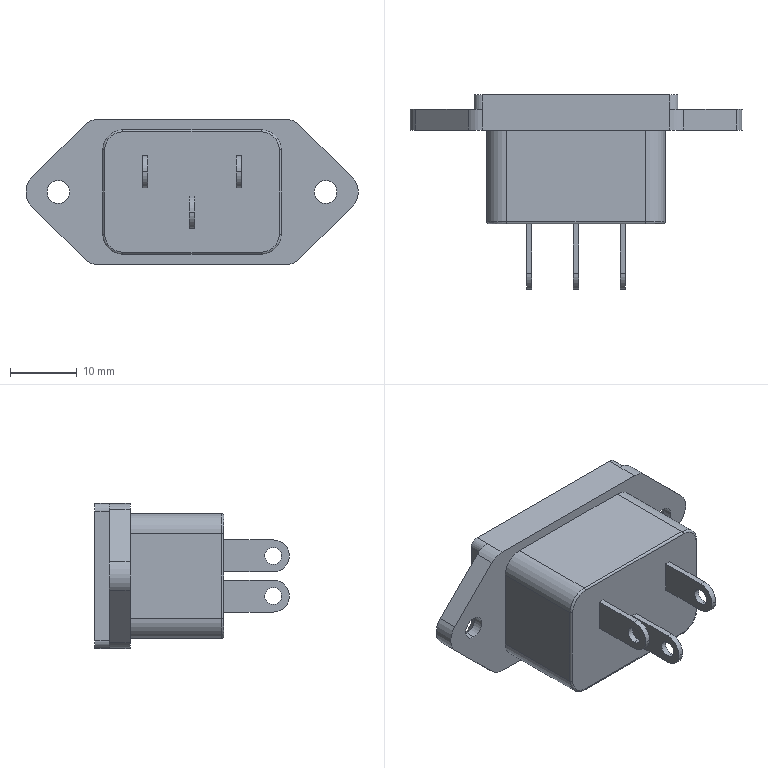Part | SolidWorks | features BaseBody 1 | 1 solid | 99 faces | box 49.7 x 29.1 x 21.7 mm | volume 6028 mm3 | plane 57 | cylinder 34 | torus 4 | cone 4 | commonest cylinder face diameters 6 x10 2.5 x6 4.8 x6 0.6 x4 2.49 x4 3.4 x4